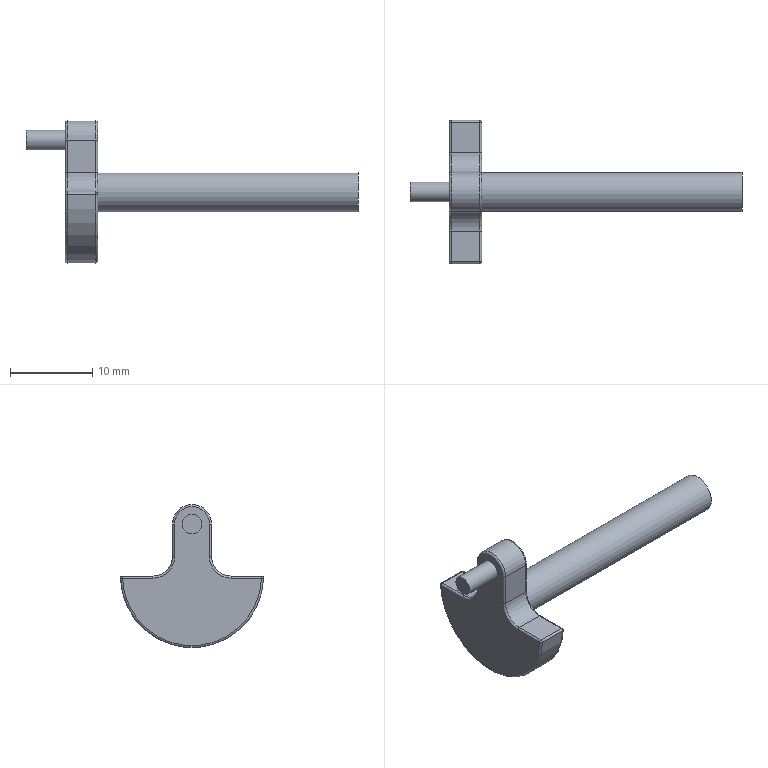Part | NX | features DATUM_CSYS 4, EXTRUDE 3, SKETCH 3, BLEND 1 | 1 solid | 36 faces | box 40.481 x 17.455 x 17.462 mm | volume 1225 mm3 | cylinder 16 | plane 8 | torus 8 | sphere 4 | commonest cylinder face diameters 0.508 x10 4.762 x3 2.381 x1 4.763 x1 17.462 x1
STEP:
#1=CARTESIAN_POINT('',(3.715,-4.762,0.));
#2=VERTEX_POINT('',#1);
#3=CARTESIAN_POINT('',(0.254,-4.762,0.));
#4=VERTEX_POINT('',#3);
#5=CARTESIAN_POINT('',(3.969,-4.762,0.));
#6=DIRECTION('',(-1.,0.,0.));
#7=VECTOR('',#6,1000.);
#8=LINE('',#5,#7);
#9=EDGE_CURVE('',#2,#4,#8,.T.);
#10=ORIENTED_EDGE('',*,*,#9,.T.);
#11=CARTESIAN_POINT('',(0.254,-8.473,0.));
#12=VERTEX_POINT('',#11);
#13=CARTESIAN_POINT('',(0.254,-4.762,0.));
#14=DIRECTION('',(0.,-1.,0.));
#15=VECTOR('',#14,1000.);
#16=LINE('',#13,#15);
#17=EDGE_CURVE('',#4,#12,#16,.T.);
#18=ORIENTED_EDGE('',*,*,#17,.T.);
#19=CARTESIAN_POINT('',(3.715,-8.473,0.));
#20=VERTEX_POINT('',#19);
#21=CARTESIAN_POINT('',(3.969,-8.473,0.));
#22=DIRECTION('',(-1.,0.,0.));
#23=VECTOR('',#22,1000.);
#24=LINE('',#21,#23);
#25=EDGE_CURVE('',#12,#20,#24,.F.);
#26=ORIENTED_EDGE('',*,*,#25,.T.);
#27=CARTESIAN_POINT('',(3.715,-4.762,0.));
#28=DIRECTION('',(0.,-1.,0.));
#29=VECTOR('',#28,1000.);
#30=LINE('',#27,#29);
#31=EDGE_CURVE('',#20,#2,#30,.F.);
#32=ORIENTED_EDGE('',*,*,#31,.T.);
#33=EDGE_LOOP('',(#10,#18,#26,#32));
#34=FACE_BOUND('',#33,.T.);
#35=CARTESIAN_POINT('',(3.969,-4.762,0.));
#36=DIRECTION('',(0.,0.,-1.));
#37=DIRECTION('',(0.,1.,0.));
#38=AXIS2_PLACEMENT_3D('',#35,#36,#37);
#39=PLANE('',#38);
#40=ADVANCED_FACE('',(#34),#39,.F.);
#41=CARTESIAN_POINT('',(0.254,-8.727,-0.2616));
#42=VERTEX_POINT('',#41);
#43=CARTESIAN_POINT('',(0.254,8.727,-0.2616));
#44=VERTEX_POINT('',#43);
#45=CARTESIAN_POINT('',(0.254,0.,0.));
#46=DIRECTION('',(1.,0.,0.));
#47=DIRECTION('',(0.,0.,-1.));
#48=AXIS2_PLACEMENT_3D('',#45,#46,#47);
#49=CIRCLE('',#48,8.731);
#50=EDGE_CURVE('',#42,#44,#49,.T.);
#51=ORIENTED_EDGE('',*,*,#50,.T.);
#52=CARTESIAN_POINT('',(3.715,8.727,-0.2616));
#53=VERTEX_POINT('',#52);
#54=CARTESIAN_POINT('',(3.969,8.727,-0.2616));
#55=DIRECTION('',(-1.,0.,0.));
#56=VECTOR('',#55,1000.);
#57=LINE('',#54,#56);
#58=EDGE_CURVE('',#44,#53,#57,.F.);
#59=ORIENTED_EDGE('',*,*,#58,.T.);
#60=CARTESIAN_POINT('',(3.715,-8.727,-0.2616));
#61=VERTEX_POINT('',#60);
#62=CARTESIAN_POINT('',(3.715,0.,0.));
#63=DIRECTION('',(1.,0.,0.));
#64=DIRECTION('',(0.,0.,-1.));
#65=AXIS2_PLACEMENT_3D('',#62,#63,#64);
#66=CIRCLE('',#65,8.731);
#67=EDGE_CURVE('',#53,#61,#66,.F.);
#68=ORIENTED_EDGE('',*,*,#67,.T.);
#69=CARTESIAN_POINT('',(3.969,-8.727,-0.2616));
#70=DIRECTION('',(-1.,0.,0.));
#71=VECTOR('',#70,1000.);
#72=LINE('',#69,#71);
#73=EDGE_CURVE('',#61,#42,#72,.T.);
#74=ORIENTED_EDGE('',*,*,#73,.T.);
#75=EDGE_LOOP('',(#51,#59,#68,#74));
#76=FACE_BOUND('',#75,.T.);
#77=CARTESIAN_POINT('',(3.969,0.,0.));
#78=DIRECTION('',(-1.,0.,0.));
#79=DIRECTION('',(0.,0.,1.));
#80=AXIS2_PLACEMENT_3D('',#77,#78,#79);
#81=CYLINDRICAL_SURFACE('',#80,8.731);
#82=ADVANCED_FACE('',(#76),#81,.T.);
#83=CARTESIAN_POINT('',(3.715,8.473,0.));
#84=VERTEX_POINT('',#83);
#85=CARTESIAN_POINT('',(0.254,8.473,0.));
#86=VERTEX_POINT('',#85);
#87=CARTESIAN_POINT('',(3.969,8.473,0.));
#88=DIRECTION('',(-1.,0.,0.));
#89=VECTOR('',#88,1000.);
#90=LINE('',#87,#89);
#91=EDGE_CURVE('',#84,#86,#90,.T.);
#92=ORIENTED_EDGE('',*,*,#91,.T.);
#93=CARTESIAN_POINT('',(0.254,4.762,0.));
#94=VERTEX_POINT('',#93);
#95=CARTESIAN_POINT('',(0.254,8.731,0.));
#96=DIRECTION('',(0.,-1.,0.));
#97=VECTOR('',#96,1000.);
#98=LINE('',#95,#97);
#99=EDGE_CURVE('',#86,#94,#98,.T.);
#100=ORIENTED_EDGE('',*,*,#99,.T.);
#101=CARTESIAN_POINT('',(3.715,4.762,0.));
#102=VERTEX_POINT('',#101);
#103=CARTESIAN_POINT('',(3.969,4.762,0.));
#104=DIRECTION('',(-1.,0.,0.));
#105=VECTOR('',#104,1000.);
#106=LINE('',#103,#105);
#107=EDGE_CURVE('',#102,#94,#106,.T.);
#108=ORIENTED_EDGE('',*,*,#107,.F.);
#109=CARTESIAN_POINT('',(3.715,8.731,0.));
#110=DIRECTION('',(0.,-1.,0.));
#111=VECTOR('',#110,1000.);
#112=LINE('',#109,#111);
#113=EDGE_CURVE('',#102,#84,#112,.F.);
#114=ORIENTED_EDGE('',*,*,#113,.T.);
#115=EDGE_LOOP('',(#92,#100,#108,#114));
#116=FACE_BOUND('',#115,.T.);
#117=CARTESIAN_POINT('',(3.969,8.731,0.));
#118=DIRECTION('',(0.,0.,-1.));
#119=DIRECTION('',(0.,1.,0.));
#120=AXIS2_PLACEMENT_3D('',#117,#118,#119);
#121=PLANE('',#120);
#122=ADVANCED_FACE('',(#116),#121,.F.);
#123=ORIENTED_EDGE('',*,*,#107,.T.);
#124=CARTESIAN_POINT('',(0.254,2.381,2.381));
#125=VERTEX_POINT('',#124);
#126=CARTESIAN_POINT('',(0.254,4.762,2.381));
#127=DIRECTION('',(1.,0.,0.));
#128=DIRECTION('',(0.,0.,-1.));
#129=AXIS2_PLACEMENT_3D('',#126,#127,#128);
#130=CIRCLE('',#129,2.381);
#131=EDGE_CURVE('',#94,#125,#130,.F.);
#132=ORIENTED_EDGE('',*,*,#131,.T.);
#133=CARTESIAN_POINT('',(3.715,2.381,2.381));
#134=VERTEX_POINT('',#133);
#135=CARTESIAN_POINT('',(3.969,2.381,2.381));
#136=DIRECTION('',(-1.,0.,0.));
#137=VECTOR('',#136,1000.);
#138=LINE('',#135,#137);
#139=EDGE_CURVE('',#134,#125,#138,.T.);
#140=ORIENTED_EDGE('',*,*,#139,.F.);
#141=CARTESIAN_POINT('',(3.715,4.762,2.381));
#142=DIRECTION('',(1.,0.,0.));
#143=DIRECTION('',(0.,0.,-1.));
#144=AXIS2_PLACEMENT_3D('',#141,#142,#143);
#145=CIRCLE('',#144,2.381);
#146=EDGE_CURVE('',#134,#102,#145,.T.);
#147=ORIENTED_EDGE('',*,*,#146,.T.);
#148=EDGE_LOOP('',(#123,#132,#140,#147));
#149=FACE_BOUND('',#148,.T.);
#150=CARTESIAN_POINT('',(3.969,4.762,2.381));
#151=DIRECTION('',(-1.,0.,0.));
#152=DIRECTION('',(0.,0.,1.));
#153=AXIS2_PLACEMENT_3D('',#150,#151,#152);
#154=CYLINDRICAL_SURFACE('',#153,2.381);
#155=ADVANCED_FACE('',(#149),#154,.F.);
#156=ORIENTED_EDGE('',*,*,#139,.T.);
#157=CARTESIAN_POINT('',(0.254,2.381,6.35));
#158=VERTEX_POINT('',#157);
#159=CARTESIAN_POINT('',(0.254,2.381,2.381));
#160=DIRECTION('',(0.,0.,1.));
#161=VECTOR('',#160,1000.);
#162=LINE('',#159,#161);
#163=EDGE_CURVE('',#125,#158,#162,.T.);
#164=ORIENTED_EDGE('',*,*,#163,.T.);
#165=CARTESIAN_POINT('',(3.715,2.381,6.35));
#166=VERTEX_POINT('',#165);
#167=CARTESIAN_POINT('',(3.969,2.381,6.35));
#168=DIRECTION('',(-1.,0.,0.));
#169=VECTOR('',#168,1000.);
#170=LINE('',#167,#169);
#171=EDGE_CURVE('',#166,#158,#170,.T.);
#172=ORIENTED_EDGE('',*,*,#171,.F.);
#173=CARTESIAN_POINT('',(3.715,2.381,2.381));
#174=DIRECTION('',(0.,0.,1.));
#175=VECTOR('',#174,1000.);
#176=LINE('',#173,#175);
#177=EDGE_CURVE('',#166,#134,#176,.F.);
#178=ORIENTED_EDGE('',*,*,#177,.T.);
#179=EDGE_LOOP('',(#156,#164,#172,#178));
#180=FACE_BOUND('',#179,.T.);
#181=CARTESIAN_POINT('',(3.969,2.381,2.381));
#182=DIRECTION('',(0.,-1.,0.));
#183=DIRECTION('',(0.,0.,-1.));
#184=AXIS2_PLACEMENT_3D('',#181,#182,#183);
#185=PLANE('',#184);
#186=ADVANCED_FACE('',(#180),#185,.F.);
#187=ORIENTED_EDGE('',*,*,#171,.T.);
#188=CARTESIAN_POINT('',(0.254,-2.381,6.35));
#189=VERTEX_POINT('',#188);
#190=CARTESIAN_POINT('',(0.254,0.,6.35));
#191=DIRECTION('',(1.,0.,0.));
#192=DIRECTION('',(0.,0.,-1.));
#193=AXIS2_PLACEMENT_3D('',#190,#191,#192);
#194=CIRCLE('',#193,2.381);
#195=EDGE_CURVE('',#158,#189,#194,.T.);
#196=ORIENTED_EDGE('',*,*,#195,.T.);
#197=CARTESIAN_POINT('',(3.715,-2.381,6.35));
#198=VERTEX_POINT('',#197);
#199=CARTESIAN_POINT('',(3.969,-2.381,6.35));
#200=DIRECTION('',(-1.,0.,0.));
#201=VECTOR('',#200,1000.);
#202=LINE('',#199,#201);
#203=EDGE_CURVE('',#198,#189,#202,.T.);
#204=ORIENTED_EDGE('',*,*,#203,.F.);
#205=CARTESIAN_POINT('',(3.715,0.,6.35));
#206=DIRECTION('',(1.,0.,0.));
#207=DIRECTION('',(0.,0.,-1.));
#208=AXIS2_PLACEMENT_3D('',#205,#206,#207);
#209=CIRCLE('',#208,2.381);
#210=EDGE_CURVE('',#198,#166,#209,.F.);
#211=ORIENTED_EDGE('',*,*,#210,.T.);
#212=EDGE_LOOP('',(#187,#196,#204,#211));
#213=FACE_BOUND('',#212,.T.);
#214=CARTESIAN_POINT('',(3.969,0.,6.35));
#215=DIRECTION('',(-1.,0.,0.));
#216=DIRECTION('',(0.,0.,1.));
#217=AXIS2_PLACEMENT_3D('',#214,#215,#216);
#218=CYLINDRICAL_SURFACE('',#217,2.381);
#219=ADVANCED_FACE('',(#213),#218,.T.);
#220=ORIENTED_EDGE('',*,*,#203,.T.);
#221=CARTESIAN_POINT('',(0.254,-2.381,2.381));
#222=VERTEX_POINT('',#221);
#223=CARTESIAN_POINT('',(0.254,-2.381,6.35));
#224=DIRECTION('',(0.,0.,-1.));
#225=VECTOR('',#224,1000.);
#226=LINE('',#223,#225);
#227=EDGE_CURVE('',#189,#222,#226,.T.);
#228=ORIENTED_EDGE('',*,*,#227,.T.);
#229=CARTESIAN_POINT('',(3.715,-2.381,2.381));
#230=VERTEX_POINT('',#229);
#231=CARTESIAN_POINT('',(3.969,-2.381,2.381));
#232=DIRECTION('',(-1.,0.,0.));
#233=VECTOR('',#232,1000.);
#234=LINE('',#231,#233);
#235=EDGE_CURVE('',#230,#222,#234,.T.);
#236=ORIENTED_EDGE('',*,*,#235,.F.);
#237=CARTESIAN_POINT('',(3.715,-2.381,6.35));
#238=DIRECTION('',(0.,0.,-1.));
#239=VECTOR('',#238,1000.);
#240=LINE('',#237,#239);
#241=EDGE_CURVE('',#230,#198,#240,.F.);
#242=ORIENTED_EDGE('',*,*,#241,.T.);
#243=EDGE_LOOP('',(#220,#228,#236,#242));
#244=FACE_BOUND('',#243,.T.);
#245=CARTESIAN_POINT('',(3.969,-2.381,6.35));
#246=DIRECTION('',(0.,1.,0.));
#247=DIRECTION('',(0.,0.,1.));
#248=AXIS2_PLACEMENT_3D('',#245,#246,#247);
#249=PLANE('',#248);
#250=ADVANCED_FACE('',(#244),#249,.F.);
#251=ORIENTED_EDGE('',*,*,#235,.T.);
#252=CARTESIAN_POINT('',(0.254,-4.762,2.381));
#253=DIRECTION('',(1.,0.,0.));
#254=DIRECTION('',(0.,0.,-1.));
#255=AXIS2_PLACEMENT_3D('',#252,#253,#254);
#256=CIRCLE('',#255,2.381);
#257=EDGE_CURVE('',#222,#4,#256,.F.);
#258=ORIENTED_EDGE('',*,*,#257,.T.);
#259=ORIENTED_EDGE('',*,*,#9,.F.);
#260=CARTESIAN_POINT('',(3.715,-4.762,2.381));
#261=DIRECTION('',(1.,0.,0.));
#262=DIRECTION('',(0.,0.,-1.));
#263=AXIS2_PLACEMENT_3D('',#260,#261,#262);
#264=CIRCLE('',#263,2.381);
#265=EDGE_CURVE('',#2,#230,#264,.T.);
#266=ORIENTED_EDGE('',*,*,#265,.T.);
#267=EDGE_LOOP('',(#251,#258,#259,#266));
#268=FACE_BOUND('',#267,.T.);
#269=CARTESIAN_POINT('',(3.969,-4.762,2.381));
#270=DIRECTION('',(-1.,0.,0.));
#271=DIRECTION('',(0.,0.,1.));
#272=AXIS2_PLACEMENT_3D('',#269,#270,#271);
#273=CYLINDRICAL_SURFACE('',#272,2.381);
#274=ADVANCED_FACE('',(#268),#273,.F.);
#275=CARTESIAN_POINT('',(3.969,-4.762,-0.254));
#276=VERTEX_POINT('',#275);
#277=CARTESIAN_POINT('',(3.969,-8.473,-0.254));
#278=VERTEX_POINT('',#277);
#279=CARTESIAN_POINT('',(3.969,-8.731,-0.254));
#280=DIRECTION('',(0.,-1.,0.));
#281=VECTOR('',#280,1000.);
#282=LINE('',#279,#281);
#283=EDGE_CURVE('',#276,#278,#282,.T.);
#284=ORIENTED_EDGE('',*,*,#283,.T.);
#285=CARTESIAN_POINT('',(3.969,8.473,-0.254));
#286=VERTEX_POINT('',#285);
#287=CARTESIAN_POINT('',(3.969,0.,0.));
#288=DIRECTION('',(1.,0.,0.));
#289=DIRECTION('',(0.,0.,-1.));
#290=AXIS2_PLACEMENT_3D('',#287,#288,#289);
#291=CIRCLE('',#290,8.477);
#292=EDGE_CURVE('',#278,#286,#291,.T.);
#293=ORIENTED_EDGE('',*,*,#292,.T.);
#294=CARTESIAN_POINT('',(3.969,4.762,-0.254));
#295=VERTEX_POINT('',#294);
#296=CARTESIAN_POINT('',(3.969,4.762,-0.254));
#297=DIRECTION('',(0.,-1.,0.));
#298=VECTOR('',#297,1000.);
#299=LINE('',#296,#298);
#300=EDGE_CURVE('',#286,#295,#299,.T.);
#301=ORIENTED_EDGE('',*,*,#300,.T.);
#302=CARTESIAN_POINT('',(3.969,2.127,2.381));
#303=VERTEX_POINT('',#302);
#304=CARTESIAN_POINT('',(3.969,4.762,2.381));
#305=DIRECTION('',(1.,0.,0.));
#306=DIRECTION('',(0.,0.,-1.));
#307=AXIS2_PLACEMENT_3D('',#304,#305,#306);
#308=CIRCLE('',#307,2.635);
#309=EDGE_CURVE('',#295,#303,#308,.F.);
#310=ORIENTED_EDGE('',*,*,#309,.T.);
#311=CARTESIAN_POINT('',(3.969,2.127,6.35));
#312=VERTEX_POINT('',#311);
#313=CARTESIAN_POINT('',(3.969,2.127,6.35));
#314=DIRECTION('',(0.,0.,1.));
#315=VECTOR('',#314,1000.);
#316=LINE('',#313,#315);
#317=EDGE_CURVE('',#303,#312,#316,.T.);
#318=ORIENTED_EDGE('',*,*,#317,.T.);
#319=CARTESIAN_POINT('',(3.969,-2.127,6.35));
#320=VERTEX_POINT('',#319);
#321=CARTESIAN_POINT('',(3.969,0.,6.35));
#322=DIRECTION('',(1.,0.,0.));
#323=DIRECTION('',(0.,0.,-1.));
#324=AXIS2_PLACEMENT_3D('',#321,#322,#323);
#325=CIRCLE('',#324,2.127);
#326=EDGE_CURVE('',#312,#320,#325,.T.);
#327=ORIENTED_EDGE('',*,*,#326,.T.);
#328=CARTESIAN_POINT('',(3.969,-2.127,2.381));
#329=VERTEX_POINT('',#328);
#330=CARTESIAN_POINT('',(3.969,-2.127,2.381));
#331=DIRECTION('',(0.,0.,-1.));
#332=VECTOR('',#331,1000.);
#333=LINE('',#330,#332);
#334=EDGE_CURVE('',#320,#329,#333,.T.);
#335=ORIENTED_EDGE('',*,*,#334,.T.);
#336=CARTESIAN_POINT('',(3.969,-4.762,2.381));
#337=DIRECTION('',(1.,0.,0.));
#338=DIRECTION('',(0.,0.,-1.));
#339=AXIS2_PLACEMENT_3D('',#336,#337,#338);
#340=CIRCLE('',#339,2.635);
#341=EDGE_CURVE('',#329,#276,#340,.F.);
#342=ORIENTED_EDGE('',*,*,#341,.T.);
#343=EDGE_LOOP('',(#284,#293,#301,#310,#318,#327,#335,#342));
#344=FACE_BOUND('',#343,.T.);
#345=CARTESIAN_POINT('',(3.969,2.381,0.));
#346=VERTEX_POINT('',#345);
#347=CARTESIAN_POINT('',(3.969,0.,0.));
#348=DIRECTION('',(1.,0.,0.));
#349=DIRECTION('',(0.,1.,0.));
#350=AXIS2_PLACEMENT_3D('',#347,#348,#349);
#351=CIRCLE('',#350,2.381);
#352=EDGE_CURVE('',#346,#346,#351,.T.);
#353=ORIENTED_EDGE('',*,*,#352,.F.);
#354=EDGE_LOOP('',(#353));
#355=FACE_BOUND('',#354,.T.);
#356=CARTESIAN_POINT('',(3.969,0.,0.));
#357=DIRECTION('',(1.,0.,0.));
#358=DIRECTION('',(0.,0.,-1.));
#359=AXIS2_PLACEMENT_3D('',#356,#357,#358);
#360=PLANE('',#359);
#361=ADVANCED_FACE('',(#344,#355),#360,.T.);
#362=CARTESIAN_POINT('',(0.,4.762,-0.254));
#363=VERTEX_POINT('',#362);
#364=CARTESIAN_POINT('',(0.,8.473,-0.254));
#365=VERTEX_POINT('',#364);
#366=CARTESIAN_POINT('',(0.,0.,-0.254));
#367=DIRECTION('',(0.,-1.,0.));
#368=VECTOR('',#367,1000.);
#369=LINE('',#366,#368);
#370=EDGE_CURVE('',#363,#365,#369,.F.);
#371=ORIENTED_EDGE('',*,*,#370,.T.);
#372=CARTESIAN_POINT('',(0.,-8.473,-0.254));
#373=VERTEX_POINT('',#372);
#374=CARTESIAN_POINT('',(0.,0.,0.));
#375=DIRECTION('',(1.,0.,0.));
#376=DIRECTION('',(0.,0.,-1.));
#377=AXIS2_PLACEMENT_3D('',#374,#375,#376);
#378=CIRCLE('',#377,8.477);
#379=EDGE_CURVE('',#365,#373,#378,.F.);
#380=ORIENTED_EDGE('',*,*,#379,.T.);
#381=CARTESIAN_POINT('',(0.,-4.762,-0.254));
#382=VERTEX_POINT('',#381);
#383=CARTESIAN_POINT('',(0.,0.,-0.254));
#384=DIRECTION('',(0.,-1.,0.));
#385=VECTOR('',#384,1000.);
#386=LINE('',#383,#385);
#387=EDGE_CURVE('',#373,#382,#386,.F.);
#388=ORIENTED_EDGE('',*,*,#387,.T.);
#389=CARTESIAN_POINT('',(0.,-2.127,2.381));
#390=VERTEX_POINT('',#389);
#391=CARTESIAN_POINT('',(0.,-4.762,2.381));
#392=DIRECTION('',(1.,0.,0.));
#393=DIRECTION('',(0.,0.,-1.));
#394=AXIS2_PLACEMENT_3D('',#391,#392,#393);
#395=CIRCLE('',#394,2.635);
#396=EDGE_CURVE('',#382,#390,#395,.T.);
#397=ORIENTED_EDGE('',*,*,#396,.T.);
#398=CARTESIAN_POINT('',(0.,-2.127,6.35));
#399=VERTEX_POINT('',#398);
#400=CARTESIAN_POINT('',(0.,-2.127,0.));
#401=DIRECTION('',(0.,0.,-1.));
#402=VECTOR('',#401,1000.);
#403=LINE('',#400,#402);
#404=EDGE_CURVE('',#390,#399,#403,.F.);
#405=ORIENTED_EDGE('',*,*,#404,.T.);
#406=CARTESIAN_POINT('',(0.,2.127,6.35));
#407=VERTEX_POINT('',#406);
#408=CARTESIAN_POINT('',(0.,0.,6.35));
#409=DIRECTION('',(1.,0.,0.));
#410=DIRECTION('',(0.,0.,-1.));
#411=AXIS2_PLACEMENT_3D('',#408,#409,#410);
#412=CIRCLE('',#411,2.127);
#413=EDGE_CURVE('',#399,#407,#412,.F.);
#414=ORIENTED_EDGE('',*,*,#413,.T.);
#415=CARTESIAN_POINT('',(0.,2.127,2.381));
#416=VERTEX_POINT('',#415);
#417=CARTESIAN_POINT('',(0.,2.127,0.));
#418=DIRECTION('',(0.,0.,1.));
#419=VECTOR('',#418,1000.);
#420=LINE('',#417,#419);
#421=EDGE_CURVE('',#407,#416,#420,.F.);
#422=ORIENTED_EDGE('',*,*,#421,.T.);
#423=CARTESIAN_POINT('',(0.,4.762,2.381));
#424=DIRECTION('',(1.,0.,0.));
#425=DIRECTION('',(0.,0.,-1.));
#426=AXIS2_PLACEMENT_3D('',#423,#424,#425);
#427=CIRCLE('',#426,2.635);
#428=EDGE_CURVE('',#416,#363,#427,.T.);
#429=ORIENTED_EDGE('',*,*,#428,.T.);
#430=EDGE_LOOP('',(#371,#380,#388,#397,#405,#414,#422,#429));
#431=FACE_BOUND('',#430,.T.);
#432=CARTESIAN_POINT('',(0.,-1.191,6.35));
#433=VERTEX_POINT('',#432);
#434=CARTESIAN_POINT('',(0.,0.,6.35));
#435=DIRECTION('',(-1.,0.,0.));
#436=DIRECTION('',(0.,-1.,0.));
#437=AXIS2_PLACEMENT_3D('',#434,#435,#436);
#438=CIRCLE('',#437,1.191);
#439=EDGE_CURVE('',#433,#433,#438,.T.);
#440=ORIENTED_EDGE('',*,*,#439,.F.);
#441=EDGE_LOOP('',(#440));
#442=FACE_BOUND('',#441,.T.);
#443=CARTESIAN_POINT('',(0.,0.,0.));
#444=DIRECTION('',(1.,0.,0.));
#445=DIRECTION('',(0.,0.,-1.));
#446=AXIS2_PLACEMENT_3D('',#443,#444,#445);
#447=PLANE('',#446);
#448=ADVANCED_FACE('',(#431,#442),#447,.F.);
#449=CARTESIAN_POINT('',(35.719,2.381,0.));
#450=VERTEX_POINT('',#449);
#451=CARTESIAN_POINT('',(35.719,0.,0.));
#452=DIRECTION('',(1.,0.,0.));
#453=DIRECTION('',(0.,1.,0.));
#454=AXIS2_PLACEMENT_3D('',#451,#452,#453);
#455=CIRCLE('',#454,2.381);
#456=EDGE_CURVE('',#450,#450,#455,.T.);
#457=ORIENTED_EDGE('',*,*,#456,.F.);
#458=EDGE_LOOP('',(#457));
#459=FACE_BOUND('',#458,.T.);
#460=ORIENTED_EDGE('',*,*,#352,.T.);
#461=EDGE_LOOP('',(#460));
#462=FACE_BOUND('',#461,.T.);
#463=CARTESIAN_POINT('',(35.719,0.,0.));
#464=DIRECTION('',(-1.,0.,0.));
#465=DIRECTION('',(0.,0.,1.));
#466=AXIS2_PLACEMENT_3D('',#463,#464,#465);
#467=CYLINDRICAL_SURFACE('',#466,2.381);
#468=ADVANCED_FACE('',(#459,#462),#467,.T.);
#469=ORIENTED_EDGE('',*,*,#456,.T.);
#470=EDGE_LOOP('',(#469));
#471=FACE_BOUND('',#470,.T.);
#472=CARTESIAN_POINT('',(35.719,0.,0.));
#473=DIRECTION('',(1.,0.,0.));
#474=DIRECTION('',(0.,0.,-1.));
#475=AXIS2_PLACEMENT_3D('',#472,#473,#474);
#476=PLANE('',#475);
#477=ADVANCED_FACE('',(#471),#476,.T.);
#478=CARTESIAN_POINT('',(-4.763,-1.191,6.35));
#479=VERTEX_POINT('',#478);
#480=CARTESIAN_POINT('',(-4.763,0.,6.35));
#481=DIRECTION('',(-1.,0.,0.));
#482=DIRECTION('',(0.,-1.,0.));
#483=AXIS2_PLACEMENT_3D('',#480,#481,#482);
#484=CIRCLE('',#483,1.191);
#485=EDGE_CURVE('',#479,#479,#484,.T.);
#486=ORIENTED_EDGE('',*,*,#485,.F.);
#487=EDGE_LOOP('',(#486));
#488=FACE_BOUND('',#487,.T.);
#489=ORIENTED_EDGE('',*,*,#439,.T.);
#490=EDGE_LOOP('',(#489));
#491=FACE_BOUND('',#490,.T.);
#492=CARTESIAN_POINT('',(-4.763,0.,6.35));
#493=DIRECTION('',(1.,0.,0.));
#494=DIRECTION('',(0.,0.,-1.));
#495=AXIS2_PLACEMENT_3D('',#492,#493,#494);
#496=CYLINDRICAL_SURFACE('',#495,1.191);
#497=ADVANCED_FACE('',(#488,#491),#496,.T.);
#498=ORIENTED_EDGE('',*,*,#485,.T.);
#499=EDGE_LOOP('',(#498));
#500=FACE_BOUND('',#499,.T.);
#501=CARTESIAN_POINT('',(-4.763,0.,6.35));
#502=DIRECTION('',(-1.,0.,0.));
#503=DIRECTION('',(0.,0.,1.));
#504=AXIS2_PLACEMENT_3D('',#501,#502,#503);
#505=PLANE('',#504);
#506=ADVANCED_FACE('',(#500),#505,.T.);
#507=CARTESIAN_POINT('',(0.254,2.127,6.35));
#508=DIRECTION('',(0.,0.,-1.));
#509=DIRECTION('',(-1.,0.,0.));
#510=AXIS2_PLACEMENT_3D('',#507,#508,#509);
#511=CIRCLE('',#510,0.254);
#512=EDGE_CURVE('',#407,#158,#511,.T.);
#513=ORIENTED_EDGE('',*,*,#512,.F.);
#514=ORIENTED_EDGE('',*,*,#413,.F.);
#515=CARTESIAN_POINT('',(0.254,-2.127,6.35));
#516=DIRECTION('',(0.,0.,-1.));
#517=DIRECTION('',(-1.,0.,0.));
#518=AXIS2_PLACEMENT_3D('',#515,#516,#517);
#519=CIRCLE('',#518,0.254);
#520=EDGE_CURVE('',#399,#189,#519,.F.);
#521=ORIENTED_EDGE('',*,*,#520,.T.);
#522=ORIENTED_EDGE('',*,*,#195,.F.);
#523=EDGE_LOOP('',(#513,#514,#521,#522));
#524=FACE_BOUND('',#523,.T.);
#525=CARTESIAN_POINT('',(0.254,0.,6.35));
#526=DIRECTION('',(1.,0.,0.));
#527=DIRECTION('',(0.,0.,-1.));
#528=AXIS2_PLACEMENT_3D('',#525,#526,#527);
#529=TOROIDAL_SURFACE('',#528,2.127,0.254);
#530=ADVANCED_FACE('',(#524),#529,.T.);
#531=ORIENTED_EDGE('',*,*,#520,.F.);
#532=ORIENTED_EDGE('',*,*,#404,.F.);
#533=CARTESIAN_POINT('',(0.254,-2.127,2.381));
#534=DIRECTION('',(0.,0.,-1.));
#535=DIRECTION('',(-1.,0.,0.));
#536=AXIS2_PLACEMENT_3D('',#533,#534,#535);
#537=CIRCLE('',#536,0.254);
#538=EDGE_CURVE('',#390,#222,#537,.F.);
#539=ORIENTED_EDGE('',*,*,#538,.T.);
#540=ORIENTED_EDGE('',*,*,#227,.F.);
#541=EDGE_LOOP('',(#531,#532,#539,#540));
#542=FACE_BOUND('',#541,.T.);
#543=CARTESIAN_POINT('',(0.254,-2.127,6.35));
#544=DIRECTION('',(0.,0.,-1.));
#545=DIRECTION('',(-1.,0.,0.));
#546=AXIS2_PLACEMENT_3D('',#543,#544,#545);
#547=CYLINDRICAL_SURFACE('',#546,0.254);
#548=ADVANCED_FACE('',(#542),#547,.T.);
#549=ORIENTED_EDGE('',*,*,#512,.T.);
#550=ORIENTED_EDGE('',*,*,#163,.F.);
#551=CARTESIAN_POINT('',(0.254,2.127,2.381));
#552=DIRECTION('',(0.,0.,-1.));
#553=DIRECTION('',(-1.,0.,0.));
#554=AXIS2_PLACEMENT_3D('',#551,#552,#553);
#555=CIRCLE('',#554,0.254);
#556=EDGE_CURVE('',#416,#125,#555,.T.);
#557=ORIENTED_EDGE('',*,*,#556,.F.);
#558=ORIENTED_EDGE('',*,*,#421,.F.);
#559=EDGE_LOOP('',(#549,#550,#557,#558));
#560=FACE_BOUND('',#559,.T.);
#561=CARTESIAN_POINT('',(0.254,2.127,2.381));
#562=DIRECTION('',(0.,0.,1.));
#563=DIRECTION('',(0.,-1.,0.));
#564=AXIS2_PLACEMENT_3D('',#561,#562,#563);
#565=CYLINDRICAL_SURFACE('',#564,0.254);
#566=ADVANCED_FACE('',(#560),#565,.T.);
#567=ORIENTED_EDGE('',*,*,#538,.F.);
#568=ORIENTED_EDGE('',*,*,#396,.F.);
#569=CARTESIAN_POINT('',(0.254,-4.762,-0.254));
#570=DIRECTION('',(0.,-1.,0.));
#571=DIRECTION('',(0.,0.,-1.));
#572=AXIS2_PLACEMENT_3D('',#569,#570,#571);
#573=CIRCLE('',#572,0.254);
#574=EDGE_CURVE('',#382,#4,#573,.F.);
#575=ORIENTED_EDGE('',*,*,#574,.T.);
#576=ORIENTED_EDGE('',*,*,#257,.F.);
#577=EDGE_LOOP('',(#567,#568,#575,#576));
#578=FACE_BOUND('',#577,.T.);
#579=CARTESIAN_POINT('',(0.254,-4.762,2.381));
#580=DIRECTION('',(1.,0.,0.));
#581=DIRECTION('',(0.,0.,-1.));
#582=AXIS2_PLACEMENT_3D('',#579,#580,#581);
#583=TOROIDAL_SURFACE('',#582,2.635,0.254);
#584=ADVANCED_FACE('',(#578),#583,.T.);
#585=CARTESIAN_POINT('',(3.715,2.127,6.35));
#586=DIRECTION('',(0.,0.,-1.));
#587=DIRECTION('',(-1.,0.,0.));
#588=AXIS2_PLACEMENT_3D('',#585,#586,#587);
#589=CIRCLE('',#588,0.254);
#590=EDGE_CURVE('',#166,#312,#589,.T.);
#591=ORIENTED_EDGE('',*,*,#590,.F.);
#592=ORIENTED_EDGE('',*,*,#210,.F.);
#593=CARTESIAN_POINT('',(3.715,-2.127,6.35));
#594=DIRECTION('',(0.,0.,-1.));
#595=DIRECTION('',(-1.,0.,0.));
#596=AXIS2_PLACEMENT_3D('',#593,#594,#595);
#597=CIRCLE('',#596,0.254);
#598=EDGE_CURVE('',#198,#320,#597,.F.);
#599=ORIENTED_EDGE('',*,*,#598,.T.);
#600=ORIENTED_EDGE('',*,*,#326,.F.);
#601=EDGE_LOOP('',(#591,#592,#599,#600));
#602=FACE_BOUND('',#601,.T.);
#603=CARTESIAN_POINT('',(3.715,0.,6.35));
#604=DIRECTION('',(1.,0.,0.));
#605=DIRECTION('',(0.,0.,-1.));
#606=AXIS2_PLACEMENT_3D('',#603,#604,#605);
#607=TOROIDAL_SURFACE('',#606,2.127,0.254);
#608=ADVANCED_FACE('',(#602),#607,.T.);
#609=ORIENTED_EDGE('',*,*,#556,.T.);
#610=ORIENTED_EDGE('',*,*,#131,.F.);
#611=CARTESIAN_POINT('',(0.254,4.762,-0.254));
#612=DIRECTION('',(0.,1.,0.));
#613=DIRECTION('',(0.,0.,1.));
#614=AXIS2_PLACEMENT_3D('',#611,#612,#613);
#615=CIRCLE('',#614,0.254);
#616=EDGE_CURVE('',#363,#94,#615,.T.);
#617=ORIENTED_EDGE('',*,*,#616,.F.);
#618=ORIENTED_EDGE('',*,*,#428,.F.);
#619=EDGE_LOOP('',(#609,#610,#617,#618));
#620=FACE_BOUND('',#619,.T.);
#621=CARTESIAN_POINT('',(0.254,4.762,2.381));
#622=DIRECTION('',(1.,0.,0.));
#623=DIRECTION('',(0.,0.,-1.));
#624=AXIS2_PLACEMENT_3D('',#621,#622,#623);
#625=TOROIDAL_SURFACE('',#624,2.635,0.254);
#626=ADVANCED_FACE('',(#620),#625,.T.);
#627=ORIENTED_EDGE('',*,*,#574,.F.);
#628=ORIENTED_EDGE('',*,*,#387,.F.);
#629=CARTESIAN_POINT('',(0.254,-8.473,-0.254));
#630=DIRECTION('',(0.,-1.,0.));
#631=DIRECTION('',(0.,0.,-1.));
#632=AXIS2_PLACEMENT_3D('',#629,#630,#631);
#633=CIRCLE('',#632,0.254);
#634=EDGE_CURVE('',#12,#373,#633,.T.);
#635=ORIENTED_EDGE('',*,*,#634,.F.);
#636=ORIENTED_EDGE('',*,*,#17,.F.);
#637=EDGE_LOOP('',(#627,#628,#635,#636));
#638=FACE_BOUND('',#637,.T.);
#639=CARTESIAN_POINT('',(0.254,-4.762,-0.254));
#640=DIRECTION('',(0.,-1.,0.));
#641=DIRECTION('',(0.,0.,-1.));
#642=AXIS2_PLACEMENT_3D('',#639,#640,#641);
#643=CYLINDRICAL_SURFACE('',#642,0.254);
#644=ADVANCED_FACE('',(#638),#643,.T.);
#645=ORIENTED_EDGE('',*,*,#598,.F.);
#646=ORIENTED_EDGE('',*,*,#241,.F.);
#647=CARTESIAN_POINT('',(3.715,-2.127,2.381));
#648=DIRECTION('',(0.,0.,-1.));
#649=DIRECTION('',(-1.,0.,0.));
#650=AXIS2_PLACEMENT_3D('',#647,#648,#649);
#651=CIRCLE('',#650,0.254);
#652=EDGE_CURVE('',#230,#329,#651,.F.);
#653=ORIENTED_EDGE('',*,*,#652,.T.);
#654=ORIENTED_EDGE('',*,*,#334,.F.);
#655=EDGE_LOOP('',(#645,#646,#653,#654));
#656=FACE_BOUND('',#655,.T.);
#657=CARTESIAN_POINT('',(3.715,-2.127,0.));
#658=DIRECTION('',(0.,0.,1.));
#659=DIRECTION('',(1.,0.,0.));
#660=AXIS2_PLACEMENT_3D('',#657,#658,#659);
#661=CYLINDRICAL_SURFACE('',#660,0.254);
#662=ADVANCED_FACE('',(#656),#661,.T.);
#663=ORIENTED_EDGE('',*,*,#590,.T.);
#664=ORIENTED_EDGE('',*,*,#317,.F.);
#665=CARTESIAN_POINT('',(3.715,2.127,2.381));
#666=DIRECTION('',(0.,0.,-1.));
#667=DIRECTION('',(-1.,0.,0.));
#668=AXIS2_PLACEMENT_3D('',#665,#666,#667);
#669=CIRCLE('',#668,0.254);
#670=EDGE_CURVE('',#134,#303,#669,.T.);
#671=ORIENTED_EDGE('',*,*,#670,.F.);
#672=ORIENTED_EDGE('',*,*,#177,.F.);
#673=EDGE_LOOP('',(#663,#664,#671,#672));
#674=FACE_BOUND('',#673,.T.);
#675=CARTESIAN_POINT('',(3.715,2.127,0.));
#676=DIRECTION('',(0.,0.,-1.));
#677=DIRECTION('',(0.,1.,0.));
#678=AXIS2_PLACEMENT_3D('',#675,#676,#677);
#679=CYLINDRICAL_SURFACE('',#678,0.254);
#680=ADVANCED_FACE('',(#674),#679,.T.);
#681=ORIENTED_EDGE('',*,*,#616,.T.);
#682=ORIENTED_EDGE('',*,*,#99,.F.);
#683=CARTESIAN_POINT('',(0.254,8.473,-0.254));
#684=DIRECTION('',(0.,1.,0.));
#685=DIRECTION('',(0.,0.,1.));
#686=AXIS2_PLACEMENT_3D('',#683,#684,#685);
#687=CIRCLE('',#686,0.254);
#688=EDGE_CURVE('',#365,#86,#687,.T.);
#689=ORIENTED_EDGE('',*,*,#688,.F.);
#690=ORIENTED_EDGE('',*,*,#370,.F.);
#691=EDGE_LOOP('',(#681,#682,#689,#690));
#692=FACE_BOUND('',#691,.T.);
#693=CARTESIAN_POINT('',(0.254,8.731,-0.254));
#694=DIRECTION('',(0.,-1.,0.));
#695=DIRECTION('',(0.,0.,-1.));
#696=AXIS2_PLACEMENT_3D('',#693,#694,#695);
#697=CYLINDRICAL_SURFACE('',#696,0.254);
#698=ADVANCED_FACE('',(#692),#697,.T.);
#699=CARTESIAN_POINT('',(0.254,-8.473,-0.254));
#700=DIRECTION('',(0.,-0.02996,0.9996));
#701=DIRECTION('',(0.,-0.9996,-0.02996));
#702=AXIS2_PLACEMENT_3D('',#699,#700,#701);
#703=CIRCLE('',#702,0.254);
#704=EDGE_CURVE('',#373,#42,#703,.T.);
#705=ORIENTED_EDGE('',*,*,#704,.F.);
#706=ORIENTED_EDGE('',*,*,#379,.F.);
#707=CARTESIAN_POINT('',(0.254,8.473,-0.254));
#708=DIRECTION('',(0.,0.02996,0.9996));
#709=DIRECTION('',(0.,-0.9996,0.02996));
#710=AXIS2_PLACEMENT_3D('',#707,#708,#709);
#711=CIRCLE('',#710,0.254);
#712=EDGE_CURVE('',#44,#365,#711,.T.);
#713=ORIENTED_EDGE('',*,*,#712,.F.);
#714=ORIENTED_EDGE('',*,*,#50,.F.);
#715=EDGE_LOOP('',(#705,#706,#713,#714));
#716=FACE_BOUND('',#715,.T.);
#717=CARTESIAN_POINT('',(0.254,0.,0.));
#718=DIRECTION('',(1.,0.,0.));
#719=DIRECTION('',(0.,0.,-1.));
#720=AXIS2_PLACEMENT_3D('',#717,#718,#719);
#721=TOROIDAL_SURFACE('',#720,8.477,0.254);
#722=ADVANCED_FACE('',(#716),#721,.T.);
#723=ORIENTED_EDGE('',*,*,#634,.T.);
#724=ORIENTED_EDGE('',*,*,#704,.T.);
#725=CARTESIAN_POINT('',(0.254,-8.473,-0.254));
#726=DIRECTION('',(-1.,0.,0.));
#727=DIRECTION('',(0.,0.,1.));
#728=AXIS2_PLACEMENT_3D('',#725,#726,#727);
#729=CIRCLE('',#728,0.254);
#730=EDGE_CURVE('',#12,#42,#729,.F.);
#731=ORIENTED_EDGE('',*,*,#730,.F.);
#732=EDGE_LOOP('',(#723,#724,#731));
#733=FACE_BOUND('',#732,.T.);
#734=CARTESIAN_POINT('',(0.254,-8.473,-0.254));
#735=DIRECTION('',(0.,0.,1.));
#736=DIRECTION('',(1.,0.,0.));
#737=AXIS2_PLACEMENT_3D('',#734,#735,#736);
#738=SPHERICAL_SURFACE('',#737,0.254);
#739=ADVANCED_FACE('',(#733),#738,.T.);
#740=ORIENTED_EDGE('',*,*,#652,.F.);
#741=ORIENTED_EDGE('',*,*,#265,.F.);
#742=CARTESIAN_POINT('',(3.715,-4.762,-0.254));
#743=DIRECTION('',(0.,-1.,0.));
#744=DIRECTION('',(0.,0.,-1.));
#745=AXIS2_PLACEMENT_3D('',#742,#743,#744);
#746=CIRCLE('',#745,0.254);
#747=EDGE_CURVE('',#2,#276,#746,.F.);
#748=ORIENTED_EDGE('',*,*,#747,.T.);
#749=ORIENTED_EDGE('',*,*,#341,.F.);
#750=EDGE_LOOP('',(#740,#741,#748,#749));
#751=FACE_BOUND('',#750,.T.);
#752=CARTESIAN_POINT('',(3.715,-4.762,2.381));
#753=DIRECTION('',(1.,0.,0.));
#754=DIRECTION('',(0.,0.,-1.));
#755=AXIS2_PLACEMENT_3D('',#752,#753,#754);
#756=TOROIDAL_SURFACE('',#755,2.635,0.254);
#757=ADVANCED_FACE('',(#751),#756,.T.);
#758=ORIENTED_EDGE('',*,*,#670,.T.);
#759=ORIENTED_EDGE('',*,*,#309,.F.);
#760=CARTESIAN_POINT('',(3.715,4.762,-0.254));
#761=DIRECTION('',(0.,1.,0.));
#762=DIRECTION('',(0.,0.,1.));
#763=AXIS2_PLACEMENT_3D('',#760,#761,#762);
#764=CIRCLE('',#763,0.254);
#765=EDGE_CURVE('',#102,#295,#764,.T.);
#766=ORIENTED_EDGE('',*,*,#765,.F.);
#767=ORIENTED_EDGE('',*,*,#146,.F.);
#768=EDGE_LOOP('',(#758,#759,#766,#767));
#769=FACE_BOUND('',#768,.T.);
#770=CARTESIAN_POINT('',(3.715,4.762,2.381));
#771=DIRECTION('',(1.,0.,0.));
#772=DIRECTION('',(0.,0.,-1.));
#773=AXIS2_PLACEMENT_3D('',#770,#771,#772);
#774=TOROIDAL_SURFACE('',#773,2.635,0.254);
#775=ADVANCED_FACE('',(#769),#774,.T.);
#776=ORIENTED_EDGE('',*,*,#712,.T.);
#777=ORIENTED_EDGE('',*,*,#688,.T.);
#778=CARTESIAN_POINT('',(0.254,8.473,-0.254));
#779=DIRECTION('',(-1.,0.,0.));
#780=DIRECTION('',(0.,0.,1.));
#781=AXIS2_PLACEMENT_3D('',#778,#779,#780);
#782=CIRCLE('',#781,0.254);
#783=EDGE_CURVE('',#44,#86,#782,.F.);
#784=ORIENTED_EDGE('',*,*,#783,.F.);
#785=EDGE_LOOP('',(#776,#777,#784));
#786=FACE_BOUND('',#785,.T.);
#787=CARTESIAN_POINT('',(0.254,8.473,-0.254));
#788=DIRECTION('',(0.,0.,1.));
#789=DIRECTION('',(1.,0.,0.));
#790=AXIS2_PLACEMENT_3D('',#787,#788,#789);
#791=SPHERICAL_SURFACE('',#790,0.254);
#792=ADVANCED_FACE('',(#786),#791,.T.);
#793=ORIENTED_EDGE('',*,*,#730,.T.);
#794=ORIENTED_EDGE('',*,*,#73,.F.);
#795=CARTESIAN_POINT('',(3.715,-8.473,-0.254));
#796=DIRECTION('',(1.,0.,0.));
#797=DIRECTION('',(0.,0.,-1.));
#798=AXIS2_PLACEMENT_3D('',#795,#796,#797);
#799=CIRCLE('',#798,0.254);
#800=EDGE_CURVE('',#20,#61,#799,.T.);
#801=ORIENTED_EDGE('',*,*,#800,.F.);
#802=ORIENTED_EDGE('',*,*,#25,.F.);
#803=EDGE_LOOP('',(#793,#794,#801,#802));
#804=FACE_BOUND('',#803,.T.);
#805=CARTESIAN_POINT('',(3.969,-8.473,-0.254));
#806=DIRECTION('',(-1.,0.,0.));
#807=DIRECTION('',(0.,0.,1.));
#808=AXIS2_PLACEMENT_3D('',#805,#806,#807);
#809=CYLINDRICAL_SURFACE('',#808,0.254);
#810=ADVANCED_FACE('',(#804),#809,.T.);
#811=ORIENTED_EDGE('',*,*,#747,.F.);
#812=ORIENTED_EDGE('',*,*,#31,.F.);
#813=CARTESIAN_POINT('',(3.715,-8.473,-0.254));
#814=DIRECTION('',(0.,-1.,0.));
#815=DIRECTION('',(0.,0.,-1.));
#816=AXIS2_PLACEMENT_3D('',#813,#814,#815);
#817=CIRCLE('',#816,0.254);
#818=EDGE_CURVE('',#278,#20,#817,.T.);
#819=ORIENTED_EDGE('',*,*,#818,.F.);
#820=ORIENTED_EDGE('',*,*,#283,.F.);
#821=EDGE_LOOP('',(#811,#812,#819,#820));
#822=FACE_BOUND('',#821,.T.);
#823=CARTESIAN_POINT('',(3.715,0.,-0.254));
#824=DIRECTION('',(0.,1.,0.));
#825=DIRECTION('',(0.,0.,1.));
#826=AXIS2_PLACEMENT_3D('',#823,#824,#825);
#827=CYLINDRICAL_SURFACE('',#826,0.254);
#828=ADVANCED_FACE('',(#822),#827,.T.);
#829=ORIENTED_EDGE('',*,*,#765,.T.);
#830=ORIENTED_EDGE('',*,*,#300,.F.);
#831=CARTESIAN_POINT('',(3.715,8.473,-0.254));
#832=DIRECTION('',(0.,1.,0.));
#833=DIRECTION('',(0.,0.,1.));
#834=AXIS2_PLACEMENT_3D('',#831,#832,#833);
#835=CIRCLE('',#834,0.254);
#836=EDGE_CURVE('',#84,#286,#835,.T.);
#837=ORIENTED_EDGE('',*,*,#836,.F.);
#838=ORIENTED_EDGE('',*,*,#113,.F.);
#839=EDGE_LOOP('',(#829,#830,#837,#838));
#840=FACE_BOUND('',#839,.T.);
#841=CARTESIAN_POINT('',(3.715,0.,-0.254));
#842=DIRECTION('',(0.,1.,0.));
#843=DIRECTION('',(0.,0.,1.));
#844=AXIS2_PLACEMENT_3D('',#841,#842,#843);
#845=CYLINDRICAL_SURFACE('',#844,0.254);
#846=ADVANCED_FACE('',(#840),#845,.T.);
#847=ORIENTED_EDGE('',*,*,#783,.T.);
#848=ORIENTED_EDGE('',*,*,#91,.F.);
#849=CARTESIAN_POINT('',(3.715,8.473,-0.254));
#850=DIRECTION('',(1.,0.,0.));
#851=DIRECTION('',(0.,0.,-1.));
#852=AXIS2_PLACEMENT_3D('',#849,#850,#851);
#853=CIRCLE('',#852,0.254);
#854=EDGE_CURVE('',#53,#84,#853,.T.);
#855=ORIENTED_EDGE('',*,*,#854,.F.);
#856=ORIENTED_EDGE('',*,*,#58,.F.);
#857=EDGE_LOOP('',(#847,#848,#855,#856));
#858=FACE_BOUND('',#857,.T.);
#859=CARTESIAN_POINT('',(3.969,8.473,-0.254));
#860=DIRECTION('',(-1.,0.,0.));
#861=DIRECTION('',(0.,0.,1.));
#862=AXIS2_PLACEMENT_3D('',#859,#860,#861);
#863=CYLINDRICAL_SURFACE('',#862,0.254);
#864=ADVANCED_FACE('',(#858),#863,.T.);
#865=ORIENTED_EDGE('',*,*,#818,.T.);
#866=ORIENTED_EDGE('',*,*,#800,.T.);
#867=CARTESIAN_POINT('',(3.715,-8.473,-0.254));
#868=DIRECTION('',(0.,-0.02996,0.9996));
#869=DIRECTION('',(0.,-0.9996,-0.02996));
#870=AXIS2_PLACEMENT_3D('',#867,#868,#869);
#871=CIRCLE('',#870,0.254);
#872=EDGE_CURVE('',#278,#61,#871,.F.);
#873=ORIENTED_EDGE('',*,*,#872,.F.);
#874=EDGE_LOOP('',(#865,#866,#873));
#875=FACE_BOUND('',#874,.T.);
#876=CARTESIAN_POINT('',(3.715,-8.473,-0.254));
#877=DIRECTION('',(0.,0.,1.));
#878=DIRECTION('',(1.,0.,0.));
#879=AXIS2_PLACEMENT_3D('',#876,#877,#878);
#880=SPHERICAL_SURFACE('',#879,0.254);
#881=ADVANCED_FACE('',(#875),#880,.T.);
#882=ORIENTED_EDGE('',*,*,#854,.T.);
#883=ORIENTED_EDGE('',*,*,#836,.T.);
#884=CARTESIAN_POINT('',(3.715,8.473,-0.254));
#885=DIRECTION('',(0.,0.02996,0.9996));
#886=DIRECTION('',(0.,-0.9996,0.02996));
#887=AXIS2_PLACEMENT_3D('',#884,#885,#886);
#888=CIRCLE('',#887,0.254);
#889=EDGE_CURVE('',#53,#286,#888,.F.);
#890=ORIENTED_EDGE('',*,*,#889,.F.);
#891=EDGE_LOOP('',(#882,#883,#890));
#892=FACE_BOUND('',#891,.T.);
#893=CARTESIAN_POINT('',(3.715,8.473,-0.254));
#894=DIRECTION('',(0.,0.,1.));
#895=DIRECTION('',(1.,0.,0.));
#896=AXIS2_PLACEMENT_3D('',#893,#894,#895);
#897=SPHERICAL_SURFACE('',#896,0.254);
#898=ADVANCED_FACE('',(#892),#897,.T.);
#899=ORIENTED_EDGE('',*,*,#872,.T.);
#900=ORIENTED_EDGE('',*,*,#67,.F.);
#901=ORIENTED_EDGE('',*,*,#889,.T.);
#902=ORIENTED_EDGE('',*,*,#292,.F.);
#903=EDGE_LOOP('',(#899,#900,#901,#902));
#904=FACE_BOUND('',#903,.T.);
#905=CARTESIAN_POINT('',(3.715,0.,0.));
#906=DIRECTION('',(1.,0.,0.));
#907=DIRECTION('',(0.,0.,-1.));
#908=AXIS2_PLACEMENT_3D('',#905,#906,#907);
#909=TOROIDAL_SURFACE('',#908,8.477,0.254);
#910=ADVANCED_FACE('',(#904),#909,.T.);
#911=CLOSED_SHELL('',(#40,#82,#122,#155,#186,#219,#250,#274,#361,#448,#468,#477,#497,#506,#530,#548,#566,#584,#608,#626,#644,#662,#680,#698,#722,#739,#757,#775,#792,#810,#828,#846,#864,#881,#898,#910));
#912=MANIFOLD_SOLID_BREP('',#911);
#913=(LENGTH_UNIT()NAMED_UNIT(*)SI_UNIT(.MILLI.,.METRE.));
#914=UNCERTAINTY_MEASURE_WITH_UNIT(LENGTH_MEASURE(0.00001),#913,'','');
#915=(NAMED_UNIT(*)PLANE_ANGLE_UNIT()SI_UNIT($,.RADIAN.));
#916=(NAMED_UNIT(*)SI_UNIT($,.STERADIAN.)SOLID_ANGLE_UNIT());
#917=(GEOMETRIC_REPRESENTATION_CONTEXT(3)GLOBAL_UNCERTAINTY_ASSIGNED_CONTEXT((#914))GLOBAL_UNIT_ASSIGNED_CONTEXT((#913,#915,#916))REPRESENTATION_CONTEXT('',''));
#918=ADVANCED_BREP_SHAPE_REPRESENTATION('',(#912),#917);